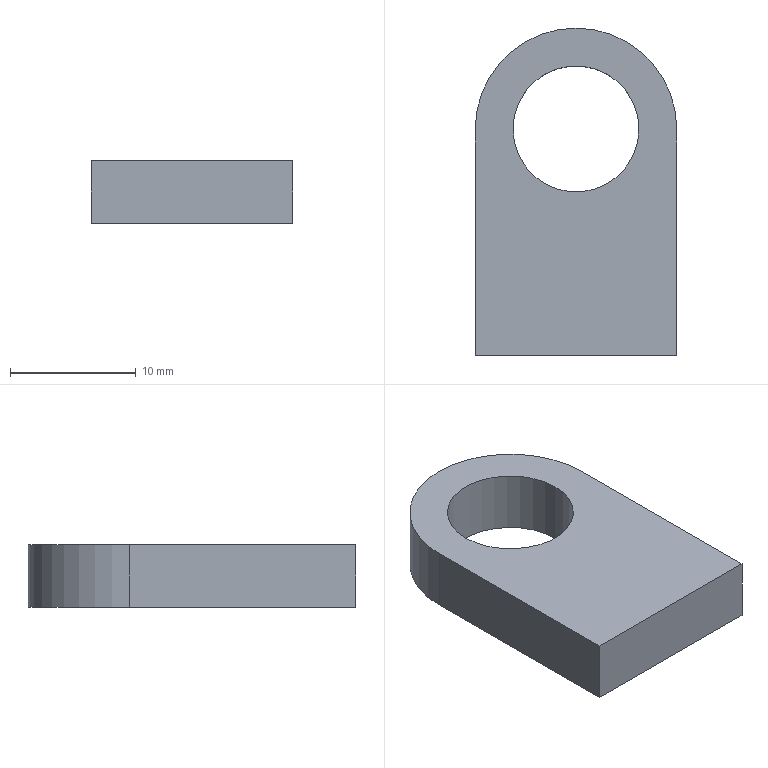Part | SolidWorks | features Extrusion 1 | 1 solid | 8 faces | box 16 x 26 x 5 mm | volume 1550 mm3 | plane 5 | cylinder 3 | commonest cylinder face diameters 10 x2 16 x1
STEP:
#1=CARTESIAN_POINT('',(-5.,18.,2.5));
#2=VERTEX_POINT('',#1);
#3=CARTESIAN_POINT('',(5.,18.,2.5));
#4=VERTEX_POINT('',#3);
#5=CARTESIAN_POINT('',(0.,18.,2.5));
#6=DIRECTION('',(0.,0.,1.));
#7=DIRECTION('',(1.,0.,0.));
#8=AXIS2_PLACEMENT_3D('',#5,#6,#7);
#9=CIRCLE('',#8,5.);
#10=EDGE_CURVE('',#2,#4,#9,.T.);
#11=ORIENTED_EDGE('',*,*,#10,.T.);
#12=CARTESIAN_POINT('',(5.,18.,-2.5));
#13=VERTEX_POINT('',#12);
#14=CARTESIAN_POINT('',(5.,18.,2.5));
#15=DIRECTION('',(0.,0.,-1.));
#16=VECTOR('',#15,1000.);
#17=LINE('',#14,#16);
#18=EDGE_CURVE('',#4,#13,#17,.T.);
#19=ORIENTED_EDGE('',*,*,#18,.T.);
#20=CARTESIAN_POINT('',(-5.,18.,-2.5));
#21=VERTEX_POINT('',#20);
#22=CARTESIAN_POINT('',(0.,18.,-2.5));
#23=DIRECTION('',(0.,0.,1.));
#24=DIRECTION('',(1.,0.,0.));
#25=AXIS2_PLACEMENT_3D('',#22,#23,#24);
#26=CIRCLE('',#25,5.);
#27=EDGE_CURVE('',#21,#13,#26,.T.);
#28=ORIENTED_EDGE('',*,*,#27,.F.);
#29=CARTESIAN_POINT('',(-5.,18.,2.5));
#30=DIRECTION('',(0.,0.,-1.));
#31=VECTOR('',#30,1000.);
#32=LINE('',#29,#31);
#33=EDGE_CURVE('',#2,#21,#32,.T.);
#34=ORIENTED_EDGE('',*,*,#33,.F.);
#35=EDGE_LOOP('',(#11,#19,#28,#34));
#36=FACE_OUTER_BOUND('',#35,.T.);
#37=CARTESIAN_POINT('',(0.,18.,2.5));
#38=DIRECTION('',(0.,0.,-1.));
#39=DIRECTION('',(-1.,0.,0.));
#40=AXIS2_PLACEMENT_3D('',#37,#38,#39);
#41=CYLINDRICAL_SURFACE('',#40,5.);
#42=ADVANCED_FACE('',(#36),#41,.F.);
#43=CARTESIAN_POINT('',(-8.,0.,2.5));
#44=VERTEX_POINT('',#43);
#45=CARTESIAN_POINT('',(8.,0.,2.5));
#46=VERTEX_POINT('',#45);
#47=CARTESIAN_POINT('',(-8.,0.,2.5));
#48=DIRECTION('',(1.,0.,0.));
#49=VECTOR('',#48,1000.);
#50=LINE('',#47,#49);
#51=EDGE_CURVE('',#44,#46,#50,.T.);
#52=ORIENTED_EDGE('',*,*,#51,.T.);
#53=CARTESIAN_POINT('',(8.,18.,2.5));
#54=VERTEX_POINT('',#53);
#55=CARTESIAN_POINT('',(8.,0.,2.5));
#56=DIRECTION('',(0.,1.,0.));
#57=VECTOR('',#56,1000.);
#58=LINE('',#55,#57);
#59=EDGE_CURVE('',#46,#54,#58,.T.);
#60=ORIENTED_EDGE('',*,*,#59,.T.);
#61=CARTESIAN_POINT('',(-8.,18.,2.5));
#62=VERTEX_POINT('',#61);
#63=CARTESIAN_POINT('',(0.,18.,2.5));
#64=DIRECTION('',(0.,0.,1.));
#65=DIRECTION('',(1.,0.,0.));
#66=AXIS2_PLACEMENT_3D('',#63,#64,#65);
#67=CIRCLE('',#66,8.);
#68=EDGE_CURVE('',#54,#62,#67,.T.);
#69=ORIENTED_EDGE('',*,*,#68,.T.);
#70=CARTESIAN_POINT('',(-8.,18.,2.5));
#71=DIRECTION('',(0.,-1.,0.));
#72=VECTOR('',#71,1000.);
#73=LINE('',#70,#72);
#74=EDGE_CURVE('',#62,#44,#73,.T.);
#75=ORIENTED_EDGE('',*,*,#74,.T.);
#76=EDGE_LOOP('',(#52,#60,#69,#75));
#77=FACE_OUTER_BOUND('',#76,.T.);
#78=ORIENTED_EDGE('',*,*,#10,.F.);
#79=CARTESIAN_POINT('',(0.,18.,2.5));
#80=DIRECTION('',(0.,0.,1.));
#81=DIRECTION('',(1.,0.,0.));
#82=AXIS2_PLACEMENT_3D('',#79,#80,#81);
#83=CIRCLE('',#82,5.);
#84=EDGE_CURVE('',#4,#2,#83,.T.);
#85=ORIENTED_EDGE('',*,*,#84,.F.);
#86=EDGE_LOOP('',(#78,#85));
#87=FACE_BOUND('',#86,.T.);
#88=CARTESIAN_POINT('',(0.,18.,2.5));
#89=DIRECTION('',(0.,0.,1.));
#90=DIRECTION('',(1.,0.,0.));
#91=AXIS2_PLACEMENT_3D('',#88,#89,#90);
#92=PLANE('',#91);
#93=ADVANCED_FACE('',(#77,#87),#92,.T.);
#94=CARTESIAN_POINT('',(-8.,0.,-2.5));
#95=VERTEX_POINT('',#94);
#96=CARTESIAN_POINT('',(8.,0.,-2.5));
#97=VERTEX_POINT('',#96);
#98=CARTESIAN_POINT('',(-8.,0.,-2.5));
#99=DIRECTION('',(1.,0.,0.));
#100=VECTOR('',#99,1000.);
#101=LINE('',#98,#100);
#102=EDGE_CURVE('',#95,#97,#101,.T.);
#103=ORIENTED_EDGE('',*,*,#102,.F.);
#104=CARTESIAN_POINT('',(-8.,18.,-2.5));
#105=VERTEX_POINT('',#104);
#106=CARTESIAN_POINT('',(-8.,18.,-2.5));
#107=DIRECTION('',(0.,-1.,0.));
#108=VECTOR('',#107,1000.);
#109=LINE('',#106,#108);
#110=EDGE_CURVE('',#105,#95,#109,.T.);
#111=ORIENTED_EDGE('',*,*,#110,.F.);
#112=CARTESIAN_POINT('',(8.,18.,-2.5));
#113=VERTEX_POINT('',#112);
#114=CARTESIAN_POINT('',(0.,18.,-2.5));
#115=DIRECTION('',(0.,0.,1.));
#116=DIRECTION('',(1.,0.,0.));
#117=AXIS2_PLACEMENT_3D('',#114,#115,#116);
#118=CIRCLE('',#117,8.);
#119=EDGE_CURVE('',#113,#105,#118,.T.);
#120=ORIENTED_EDGE('',*,*,#119,.F.);
#121=CARTESIAN_POINT('',(8.,0.,-2.5));
#122=DIRECTION('',(0.,1.,0.));
#123=VECTOR('',#122,1000.);
#124=LINE('',#121,#123);
#125=EDGE_CURVE('',#97,#113,#124,.T.);
#126=ORIENTED_EDGE('',*,*,#125,.F.);
#127=EDGE_LOOP('',(#103,#111,#120,#126));
#128=FACE_OUTER_BOUND('',#127,.T.);
#129=ORIENTED_EDGE('',*,*,#27,.T.);
#130=CARTESIAN_POINT('',(0.,18.,-2.5));
#131=DIRECTION('',(0.,0.,1.));
#132=DIRECTION('',(1.,0.,0.));
#133=AXIS2_PLACEMENT_3D('',#130,#131,#132);
#134=CIRCLE('',#133,5.);
#135=EDGE_CURVE('',#13,#21,#134,.T.);
#136=ORIENTED_EDGE('',*,*,#135,.T.);
#137=EDGE_LOOP('',(#129,#136));
#138=FACE_BOUND('',#137,.T.);
#139=CARTESIAN_POINT('',(0.,18.,-2.5));
#140=DIRECTION('',(0.,0.,1.));
#141=DIRECTION('',(1.,0.,0.));
#142=AXIS2_PLACEMENT_3D('',#139,#140,#141);
#143=PLANE('',#142);
#144=ADVANCED_FACE('',(#128,#138),#143,.F.);
#145=ORIENTED_EDGE('',*,*,#102,.T.);
#146=CARTESIAN_POINT('',(8.,0.,2.5));
#147=DIRECTION('',(0.,0.,-1.));
#148=VECTOR('',#147,1000.);
#149=LINE('',#146,#148);
#150=EDGE_CURVE('',#46,#97,#149,.T.);
#151=ORIENTED_EDGE('',*,*,#150,.F.);
#152=ORIENTED_EDGE('',*,*,#51,.F.);
#153=CARTESIAN_POINT('',(-8.,0.,2.5));
#154=DIRECTION('',(0.,0.,-1.));
#155=VECTOR('',#154,1000.);
#156=LINE('',#153,#155);
#157=EDGE_CURVE('',#44,#95,#156,.T.);
#158=ORIENTED_EDGE('',*,*,#157,.T.);
#159=EDGE_LOOP('',(#145,#151,#152,#158));
#160=FACE_OUTER_BOUND('',#159,.T.);
#161=CARTESIAN_POINT('',(-8.,0.,2.5));
#162=DIRECTION('',(0.,1.,0.));
#163=DIRECTION('',(-1.,0.,0.));
#164=AXIS2_PLACEMENT_3D('',#161,#162,#163);
#165=PLANE('',#164);
#166=ADVANCED_FACE('',(#160),#165,.F.);
#167=ORIENTED_EDGE('',*,*,#125,.T.);
#168=CARTESIAN_POINT('',(8.,18.,2.5));
#169=DIRECTION('',(0.,0.,-1.));
#170=VECTOR('',#169,1000.);
#171=LINE('',#168,#170);
#172=EDGE_CURVE('',#54,#113,#171,.T.);
#173=ORIENTED_EDGE('',*,*,#172,.F.);
#174=ORIENTED_EDGE('',*,*,#59,.F.);
#175=ORIENTED_EDGE('',*,*,#150,.T.);
#176=EDGE_LOOP('',(#167,#173,#174,#175));
#177=FACE_OUTER_BOUND('',#176,.T.);
#178=CARTESIAN_POINT('',(8.,0.,2.5));
#179=DIRECTION('',(-1.,0.,0.));
#180=DIRECTION('',(0.,0.,1.));
#181=AXIS2_PLACEMENT_3D('',#178,#179,#180);
#182=PLANE('',#181);
#183=ADVANCED_FACE('',(#177),#182,.F.);
#184=ORIENTED_EDGE('',*,*,#119,.T.);
#185=CARTESIAN_POINT('',(-8.,18.,2.5));
#186=DIRECTION('',(0.,0.,-1.));
#187=VECTOR('',#186,1000.);
#188=LINE('',#185,#187);
#189=EDGE_CURVE('',#62,#105,#188,.T.);
#190=ORIENTED_EDGE('',*,*,#189,.F.);
#191=ORIENTED_EDGE('',*,*,#68,.F.);
#192=ORIENTED_EDGE('',*,*,#172,.T.);
#193=EDGE_LOOP('',(#184,#190,#191,#192));
#194=FACE_OUTER_BOUND('',#193,.T.);
#195=CARTESIAN_POINT('',(0.,18.,2.5));
#196=DIRECTION('',(0.,0.,-1.));
#197=DIRECTION('',(-1.,0.,0.));
#198=AXIS2_PLACEMENT_3D('',#195,#196,#197);
#199=CYLINDRICAL_SURFACE('',#198,8.);
#200=ADVANCED_FACE('',(#194),#199,.T.);
#201=ORIENTED_EDGE('',*,*,#110,.T.);
#202=ORIENTED_EDGE('',*,*,#157,.F.);
#203=ORIENTED_EDGE('',*,*,#74,.F.);
#204=ORIENTED_EDGE('',*,*,#189,.T.);
#205=EDGE_LOOP('',(#201,#202,#203,#204));
#206=FACE_OUTER_BOUND('',#205,.T.);
#207=CARTESIAN_POINT('',(-8.,18.,2.5));
#208=DIRECTION('',(1.,0.,0.));
#209=DIRECTION('',(0.,1.,0.));
#210=AXIS2_PLACEMENT_3D('',#207,#208,#209);
#211=PLANE('',#210);
#212=ADVANCED_FACE('',(#206),#211,.F.);
#213=ORIENTED_EDGE('',*,*,#18,.F.);
#214=ORIENTED_EDGE('',*,*,#84,.T.);
#215=ORIENTED_EDGE('',*,*,#33,.T.);
#216=ORIENTED_EDGE('',*,*,#135,.F.);
#217=EDGE_LOOP('',(#213,#214,#215,#216));
#218=FACE_OUTER_BOUND('',#217,.T.);
#219=CARTESIAN_POINT('',(0.,18.,2.5));
#220=DIRECTION('',(0.,0.,-1.));
#221=DIRECTION('',(-1.,0.,0.));
#222=AXIS2_PLACEMENT_3D('',#219,#220,#221);
#223=CYLINDRICAL_SURFACE('',#222,5.);
#224=ADVANCED_FACE('',(#218),#223,.F.);
#225=CLOSED_SHELL('',(#42,#93,#144,#166,#183,#200,#212,#224));
#226=MANIFOLD_SOLID_BREP('',#225);
#227=CARTESIAN_POINT('',(0.,0.,0.));
#228=DIRECTION('',(0.,0.,1.));
#229=DIRECTION('',(1.,0.,0.));
#230=AXIS2_PLACEMENT_3D('',#227,#228,#229);
#231=(LENGTH_UNIT()NAMED_UNIT(*)SI_UNIT(.MILLI.,.METRE.));
#232=UNCERTAINTY_MEASURE_WITH_UNIT(LENGTH_MEASURE(0.00001),#231,'','');
#233=(NAMED_UNIT(*)PLANE_ANGLE_UNIT()SI_UNIT($,.RADIAN.));
#234=(NAMED_UNIT(*)SI_UNIT($,.STERADIAN.)SOLID_ANGLE_UNIT());
#235=(GEOMETRIC_REPRESENTATION_CONTEXT(3)GLOBAL_UNCERTAINTY_ASSIGNED_CONTEXT((#232))GLOBAL_UNIT_ASSIGNED_CONTEXT((#231,#233,#234))REPRESENTATION_CONTEXT('',''));
#236=ADVANCED_BREP_SHAPE_REPRESENTATION('',(#226,#230),#235);